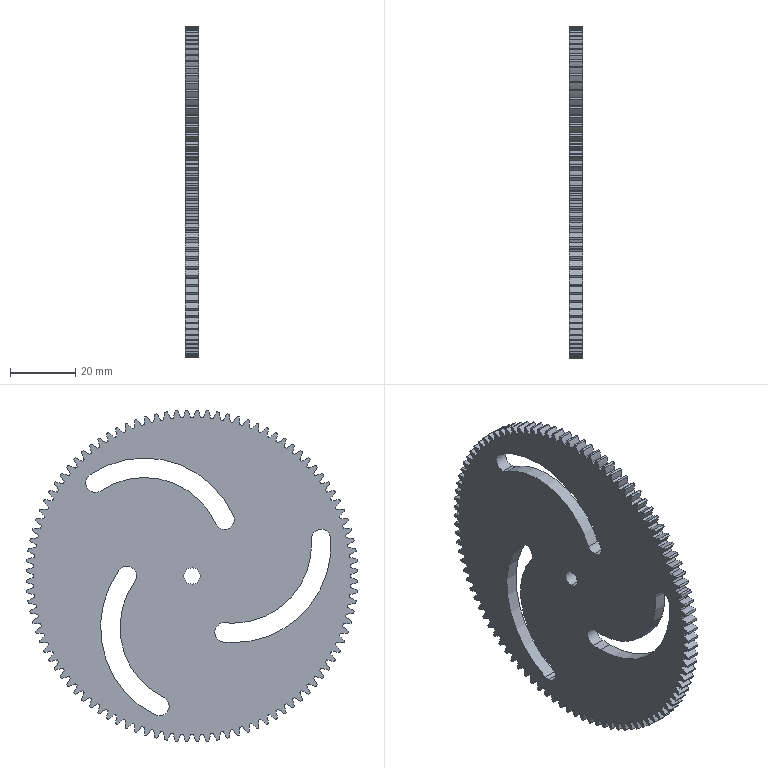Part | SolidWorks | features BaseBody 1 | 1 solid | 426 faces | box 4 x 101.968 x 101.968 mm | volume 27433 mm3 | cylinder 424 | plane 2 | commonest cylinder face diameters 40 x204 97.498 x101 102 x100 6 x9 48 x4 60 x4